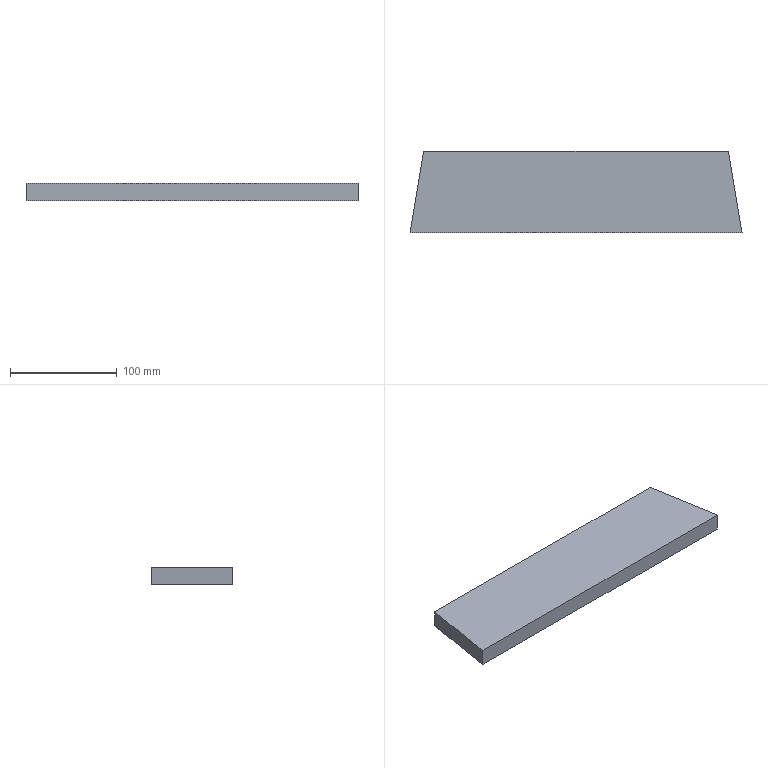Part | SolidWorks | features BaseBody 1 | 1 solid | 6 faces | box 310.603 x 76.2 x 16 mm | volume 363141 mm3 | plane 6
STEP:
#1=CARTESIAN_POINT('',(280.894,-28.252,0.));
#2=VERTEX_POINT('',#1);
#3=CARTESIAN_POINT('',(268.142,47.948,0.));
#4=VERTEX_POINT('',#3);
#5=CARTESIAN_POINT('',(280.894,-28.252,0.));
#6=DIRECTION('',(-0.165,0.9863,0.));
#7=VECTOR('',#6,1000.);
#8=LINE('',#5,#7);
#9=EDGE_CURVE('',#2,#4,#8,.T.);
#10=ORIENTED_EDGE('',*,*,#9,.F.);
#11=CARTESIAN_POINT('',(-29.709,-28.252,0.));
#12=VERTEX_POINT('',#11);
#13=CARTESIAN_POINT('',(125.592,-28.252,0.));
#14=DIRECTION('',(1.,0.,0.));
#15=VECTOR('',#14,1000.);
#16=LINE('',#13,#15);
#17=EDGE_CURVE('',#12,#2,#16,.T.);
#18=ORIENTED_EDGE('',*,*,#17,.F.);
#19=CARTESIAN_POINT('',(-16.958,47.948,0.));
#20=VERTEX_POINT('',#19);
#21=CARTESIAN_POINT('',(-16.958,47.948,0.));
#22=DIRECTION('',(-0.165,-0.9863,0.));
#23=VECTOR('',#22,1000.);
#24=LINE('',#21,#23);
#25=EDGE_CURVE('',#20,#12,#24,.T.);
#26=ORIENTED_EDGE('',*,*,#25,.F.);
#27=CARTESIAN_POINT('',(125.592,47.948,0.));
#28=DIRECTION('',(-1.,0.,0.));
#29=VECTOR('',#28,1000.);
#30=LINE('',#27,#29);
#31=EDGE_CURVE('',#4,#20,#30,.T.);
#32=ORIENTED_EDGE('',*,*,#31,.F.);
#33=EDGE_LOOP('',(#10,#18,#26,#32));
#34=FACE_OUTER_BOUND('',#33,.T.);
#35=CARTESIAN_POINT('',(125.592,8.552,0.));
#36=DIRECTION('',(0.,0.,1.));
#37=DIRECTION('',(1.,0.,0.));
#38=AXIS2_PLACEMENT_3D('',#35,#36,#37);
#39=PLANE('',#38);
#40=ADVANCED_FACE('',(#34),#39,.F.);
#41=ORIENTED_EDGE('',*,*,#31,.T.);
#42=CARTESIAN_POINT('',(-16.958,47.948,16.));
#43=VERTEX_POINT('',#42);
#44=CARTESIAN_POINT('',(-16.958,47.948,0.));
#45=DIRECTION('',(0.,0.,1.));
#46=VECTOR('',#45,1000.);
#47=LINE('',#44,#46);
#48=EDGE_CURVE('',#20,#43,#47,.T.);
#49=ORIENTED_EDGE('',*,*,#48,.T.);
#50=CARTESIAN_POINT('',(268.142,47.948,16.));
#51=VERTEX_POINT('',#50);
#52=CARTESIAN_POINT('',(-16.958,47.948,16.));
#53=DIRECTION('',(1.,0.,0.));
#54=VECTOR('',#53,1000.);
#55=LINE('',#52,#54);
#56=EDGE_CURVE('',#43,#51,#55,.T.);
#57=ORIENTED_EDGE('',*,*,#56,.T.);
#58=CARTESIAN_POINT('',(268.142,47.948,0.));
#59=DIRECTION('',(0.,0.,-1.));
#60=VECTOR('',#59,1000.);
#61=LINE('',#58,#60);
#62=EDGE_CURVE('',#51,#4,#61,.T.);
#63=ORIENTED_EDGE('',*,*,#62,.T.);
#64=EDGE_LOOP('',(#41,#49,#57,#63));
#65=FACE_OUTER_BOUND('',#64,.T.);
#66=CARTESIAN_POINT('',(-16.958,47.948,0.));
#67=DIRECTION('',(0.,1.,0.));
#68=DIRECTION('',(-1.,0.,0.));
#69=AXIS2_PLACEMENT_3D('',#66,#67,#68);
#70=PLANE('',#69);
#71=ADVANCED_FACE('',(#65),#70,.T.);
#72=ORIENTED_EDGE('',*,*,#9,.T.);
#73=ORIENTED_EDGE('',*,*,#62,.F.);
#74=CARTESIAN_POINT('',(280.894,-28.252,16.));
#75=VERTEX_POINT('',#74);
#76=CARTESIAN_POINT('',(268.142,47.948,16.));
#77=DIRECTION('',(0.165,-0.9863,0.));
#78=VECTOR('',#77,1000.);
#79=LINE('',#76,#78);
#80=EDGE_CURVE('',#51,#75,#79,.T.);
#81=ORIENTED_EDGE('',*,*,#80,.T.);
#82=CARTESIAN_POINT('',(280.894,-28.252,0.));
#83=DIRECTION('',(0.,0.,-1.));
#84=VECTOR('',#83,1000.);
#85=LINE('',#82,#84);
#86=EDGE_CURVE('',#75,#2,#85,.T.);
#87=ORIENTED_EDGE('',*,*,#86,.T.);
#88=EDGE_LOOP('',(#72,#73,#81,#87));
#89=FACE_OUTER_BOUND('',#88,.T.);
#90=CARTESIAN_POINT('',(268.142,47.948,0.));
#91=DIRECTION('',(0.9863,0.165,0.));
#92=DIRECTION('',(-0.165,0.9863,0.));
#93=AXIS2_PLACEMENT_3D('',#90,#91,#92);
#94=PLANE('',#93);
#95=ADVANCED_FACE('',(#89),#94,.T.);
#96=ORIENTED_EDGE('',*,*,#17,.T.);
#97=ORIENTED_EDGE('',*,*,#86,.F.);
#98=CARTESIAN_POINT('',(-29.709,-28.252,16.));
#99=VERTEX_POINT('',#98);
#100=CARTESIAN_POINT('',(280.894,-28.252,16.));
#101=DIRECTION('',(-1.,0.,0.));
#102=VECTOR('',#101,1000.);
#103=LINE('',#100,#102);
#104=EDGE_CURVE('',#75,#99,#103,.T.);
#105=ORIENTED_EDGE('',*,*,#104,.T.);
#106=CARTESIAN_POINT('',(-29.709,-28.252,0.));
#107=DIRECTION('',(0.,0.,-1.));
#108=VECTOR('',#107,1000.);
#109=LINE('',#106,#108);
#110=EDGE_CURVE('',#99,#12,#109,.T.);
#111=ORIENTED_EDGE('',*,*,#110,.T.);
#112=EDGE_LOOP('',(#96,#97,#105,#111));
#113=FACE_OUTER_BOUND('',#112,.T.);
#114=CARTESIAN_POINT('',(280.894,-28.252,0.));
#115=DIRECTION('',(0.,-1.,0.));
#116=DIRECTION('',(1.,0.,0.));
#117=AXIS2_PLACEMENT_3D('',#114,#115,#116);
#118=PLANE('',#117);
#119=ADVANCED_FACE('',(#113),#118,.T.);
#120=ORIENTED_EDGE('',*,*,#25,.T.);
#121=ORIENTED_EDGE('',*,*,#110,.F.);
#122=CARTESIAN_POINT('',(-29.709,-28.252,16.));
#123=DIRECTION('',(0.165,0.9863,0.));
#124=VECTOR('',#123,1000.);
#125=LINE('',#122,#124);
#126=EDGE_CURVE('',#99,#43,#125,.T.);
#127=ORIENTED_EDGE('',*,*,#126,.T.);
#128=ORIENTED_EDGE('',*,*,#48,.F.);
#129=EDGE_LOOP('',(#120,#121,#127,#128));
#130=FACE_OUTER_BOUND('',#129,.T.);
#131=CARTESIAN_POINT('',(-29.709,-28.252,0.));
#132=DIRECTION('',(-0.9863,0.165,0.));
#133=DIRECTION('',(-0.165,-0.9863,0.));
#134=AXIS2_PLACEMENT_3D('',#131,#132,#133);
#135=PLANE('',#134);
#136=ADVANCED_FACE('',(#130),#135,.T.);
#137=ORIENTED_EDGE('',*,*,#126,.F.);
#138=ORIENTED_EDGE('',*,*,#104,.F.);
#139=ORIENTED_EDGE('',*,*,#80,.F.);
#140=ORIENTED_EDGE('',*,*,#56,.F.);
#141=EDGE_LOOP('',(#137,#138,#139,#140));
#142=FACE_OUTER_BOUND('',#141,.T.);
#143=CARTESIAN_POINT('',(125.592,8.552,16.));
#144=DIRECTION('',(0.,0.,1.));
#145=DIRECTION('',(1.,0.,0.));
#146=AXIS2_PLACEMENT_3D('',#143,#144,#145);
#147=PLANE('',#146);
#148=ADVANCED_FACE('',(#142),#147,.T.);
#149=CLOSED_SHELL('',(#40,#71,#95,#119,#136,#148));
#150=MANIFOLD_SOLID_BREP('',#149);
#151=CARTESIAN_POINT('',(0.,0.,0.));
#152=DIRECTION('',(0.,0.,1.));
#153=DIRECTION('',(1.,0.,0.));
#154=AXIS2_PLACEMENT_3D('',#151,#152,#153);
#155=(LENGTH_UNIT()NAMED_UNIT(*)SI_UNIT(.MILLI.,.METRE.));
#156=UNCERTAINTY_MEASURE_WITH_UNIT(LENGTH_MEASURE(0.00001),#155,'','');
#157=(NAMED_UNIT(*)PLANE_ANGLE_UNIT()SI_UNIT($,.RADIAN.));
#158=(NAMED_UNIT(*)SI_UNIT($,.STERADIAN.)SOLID_ANGLE_UNIT());
#159=(GEOMETRIC_REPRESENTATION_CONTEXT(3)GLOBAL_UNCERTAINTY_ASSIGNED_CONTEXT((#156))GLOBAL_UNIT_ASSIGNED_CONTEXT((#155,#157,#158))REPRESENTATION_CONTEXT('',''));
#160=ADVANCED_BREP_SHAPE_REPRESENTATION('',(#150,#154),#159);